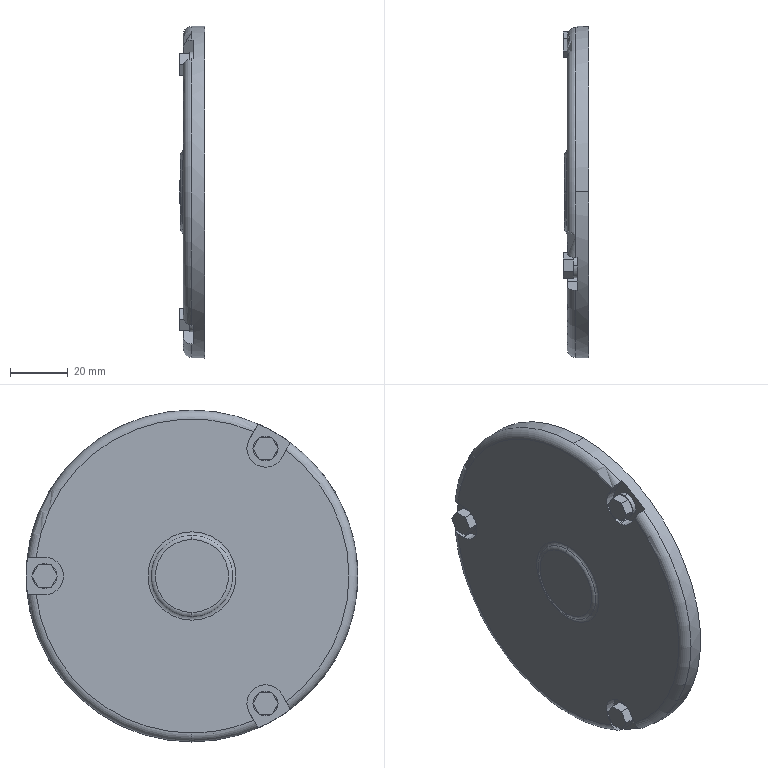Part | STEP file | G3L22N30-MM02TNNTNXH6-Part-7 | 1 solid | 89 faces | box 9 x 114.97 x 114.97 mm | volume 76875 mm3 | plane 69 | cylinder 10 | torus 8 | cone 2 | commonest cylinder face diameters 8.5 x6 13 x4